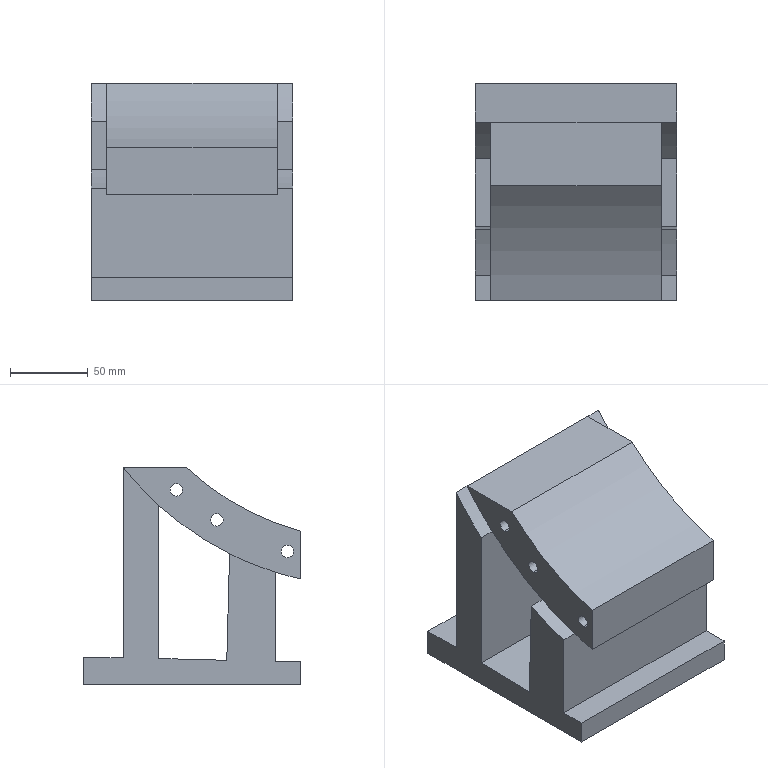Part | SolidWorks | features Cut 4, Extrusion 1, ICE 1 | 1 solid | 29 faces | box 130 x 140 x 140 mm | volume 1223723 mm3 | plane 16 | cylinder 13 | commonest cylinder face diameters 8 x6 406.59 x6 346.59 x1
STEP:
#1=CARTESIAN_POINT('',(120.,98.538,81.808));
#2=VERTEX_POINT('',#1);
#3=CARTESIAN_POINT('',(120.,98.538,89.808));
#4=VERTEX_POINT('',#3);
#5=CARTESIAN_POINT('',(120.,98.538,85.808));
#6=DIRECTION('',(-1.,0.,0.));
#7=DIRECTION('',(0.,0.,1.));
#8=AXIS2_PLACEMENT_3D('',#5,#6,#7);
#9=CIRCLE('',#8,4.);
#10=EDGE_CURVE('',#2,#4,#9,.T.);
#11=ORIENTED_EDGE('',*,*,#10,.F.);
#12=CARTESIAN_POINT('',(10.,98.538,81.808));
#13=VERTEX_POINT('',#12);
#14=CARTESIAN_POINT('',(130.,98.538,81.808));
#15=DIRECTION('',(-1.,0.,0.));
#16=VECTOR('',#15,1000.);
#17=LINE('',#14,#16);
#18=EDGE_CURVE('',#2,#13,#17,.T.);
#19=ORIENTED_EDGE('',*,*,#18,.T.);
#20=CARTESIAN_POINT('',(10.,98.538,89.808));
#21=VERTEX_POINT('',#20);
#22=CARTESIAN_POINT('',(10.,98.538,85.808));
#23=DIRECTION('',(-1.,0.,0.));
#24=DIRECTION('',(0.,0.,1.));
#25=AXIS2_PLACEMENT_3D('',#22,#23,#24);
#26=CIRCLE('',#25,4.);
#27=EDGE_CURVE('',#13,#21,#26,.T.);
#28=ORIENTED_EDGE('',*,*,#27,.T.);
#29=CARTESIAN_POINT('',(130.,98.538,89.808));
#30=DIRECTION('',(-1.,0.,0.));
#31=VECTOR('',#30,1000.);
#32=LINE('',#29,#31);
#33=EDGE_CURVE('',#4,#21,#32,.T.);
#34=ORIENTED_EDGE('',*,*,#33,.F.);
#35=EDGE_LOOP('',(#11,#19,#28,#34));
#36=FACE_OUTER_BOUND('',#35,.T.);
#37=CARTESIAN_POINT('',(130.,98.538,85.808));
#38=DIRECTION('',(-1.,0.,0.));
#39=DIRECTION('',(0.,0.,1.));
#40=AXIS2_PLACEMENT_3D('',#37,#38,#39);
#41=CYLINDRICAL_SURFACE('',#40,4.);
#42=ADVANCED_FACE('',(#36),#41,.F.);
#43=CARTESIAN_POINT('',(120.,143.974,102.133));
#44=VERTEX_POINT('',#43);
#45=CARTESIAN_POINT('',(120.,143.974,110.133));
#46=VERTEX_POINT('',#45);
#47=CARTESIAN_POINT('',(120.,143.974,106.133));
#48=DIRECTION('',(-1.,0.,0.));
#49=DIRECTION('',(0.,0.,1.));
#50=AXIS2_PLACEMENT_3D('',#47,#48,#49);
#51=CIRCLE('',#50,4.);
#52=EDGE_CURVE('',#44,#46,#51,.T.);
#53=ORIENTED_EDGE('',*,*,#52,.F.);
#54=CARTESIAN_POINT('',(10.,143.974,102.133));
#55=VERTEX_POINT('',#54);
#56=CARTESIAN_POINT('',(130.,143.974,102.133));
#57=DIRECTION('',(-1.,0.,0.));
#58=VECTOR('',#57,1000.);
#59=LINE('',#56,#58);
#60=EDGE_CURVE('',#44,#55,#59,.T.);
#61=ORIENTED_EDGE('',*,*,#60,.T.);
#62=CARTESIAN_POINT('',(10.,143.974,110.133));
#63=VERTEX_POINT('',#62);
#64=CARTESIAN_POINT('',(10.,143.974,106.133));
#65=DIRECTION('',(-1.,0.,0.));
#66=DIRECTION('',(0.,0.,1.));
#67=AXIS2_PLACEMENT_3D('',#64,#65,#66);
#68=CIRCLE('',#67,4.);
#69=EDGE_CURVE('',#55,#63,#68,.T.);
#70=ORIENTED_EDGE('',*,*,#69,.T.);
#71=CARTESIAN_POINT('',(130.,143.974,110.133));
#72=DIRECTION('',(-1.,0.,0.));
#73=VECTOR('',#72,1000.);
#74=LINE('',#71,#73);
#75=EDGE_CURVE('',#46,#63,#74,.T.);
#76=ORIENTED_EDGE('',*,*,#75,.F.);
#77=EDGE_LOOP('',(#53,#61,#70,#76));
#78=FACE_OUTER_BOUND('',#77,.T.);
#79=CARTESIAN_POINT('',(130.,143.974,106.133));
#80=DIRECTION('',(-1.,0.,0.));
#81=DIRECTION('',(0.,0.,1.));
#82=AXIS2_PLACEMENT_3D('',#79,#80,#81);
#83=CYLINDRICAL_SURFACE('',#82,4.);
#84=ADVANCED_FACE('',(#78),#83,.F.);
#85=CARTESIAN_POINT('',(120.,170.036,121.519));
#86=VERTEX_POINT('',#85);
#87=CARTESIAN_POINT('',(120.,170.036,129.519));
#88=VERTEX_POINT('',#87);
#89=CARTESIAN_POINT('',(120.,170.036,125.519));
#90=DIRECTION('',(-1.,0.,0.));
#91=DIRECTION('',(0.,0.,1.));
#92=AXIS2_PLACEMENT_3D('',#89,#90,#91);
#93=CIRCLE('',#92,4.);
#94=EDGE_CURVE('',#86,#88,#93,.T.);
#95=ORIENTED_EDGE('',*,*,#94,.F.);
#96=CARTESIAN_POINT('',(10.,170.036,121.519));
#97=VERTEX_POINT('',#96);
#98=CARTESIAN_POINT('',(130.,170.036,121.519));
#99=DIRECTION('',(-1.,0.,0.));
#100=VECTOR('',#99,1000.);
#101=LINE('',#98,#100);
#102=EDGE_CURVE('',#86,#97,#101,.T.);
#103=ORIENTED_EDGE('',*,*,#102,.T.);
#104=CARTESIAN_POINT('',(10.,170.036,129.519));
#105=VERTEX_POINT('',#104);
#106=CARTESIAN_POINT('',(10.,170.036,125.519));
#107=DIRECTION('',(-1.,0.,0.));
#108=DIRECTION('',(0.,0.,1.));
#109=AXIS2_PLACEMENT_3D('',#106,#107,#108);
#110=CIRCLE('',#109,4.);
#111=EDGE_CURVE('',#97,#105,#110,.T.);
#112=ORIENTED_EDGE('',*,*,#111,.T.);
#113=CARTESIAN_POINT('',(130.,170.036,129.519));
#114=DIRECTION('',(-1.,0.,0.));
#115=VECTOR('',#114,1000.);
#116=LINE('',#113,#115);
#117=EDGE_CURVE('',#88,#105,#116,.T.);
#118=ORIENTED_EDGE('',*,*,#117,.F.);
#119=EDGE_LOOP('',(#95,#103,#112,#118));
#120=FACE_OUTER_BOUND('',#119,.T.);
#121=CARTESIAN_POINT('',(130.,170.036,125.519));
#122=DIRECTION('',(-1.,0.,0.));
#123=DIRECTION('',(0.,0.,1.));
#124=AXIS2_PLACEMENT_3D('',#121,#122,#123);
#125=CYLINDRICAL_SURFACE('',#124,4.);
#126=ADVANCED_FACE('',(#120),#125,.F.);
#127=CARTESIAN_POINT('',(10.,90.,68.082));
#128=VERTEX_POINT('',#127);
#129=CARTESIAN_POINT('',(10.,90.,98.982));
#130=VERTEX_POINT('',#129);
#131=CARTESIAN_POINT('',(10.,90.,98.982));
#132=DIRECTION('',(0.,0.,1.));
#133=VECTOR('',#132,1000.);
#134=LINE('',#131,#133);
#135=EDGE_CURVE('',#128,#130,#134,.T.);
#136=ORIENTED_EDGE('',*,*,#135,.F.);
#137=CARTESIAN_POINT('',(120.,90.,68.082));
#138=VERTEX_POINT('',#137);
#139=CARTESIAN_POINT('',(0.,90.,68.082));
#140=DIRECTION('',(1.,0.,0.));
#141=VECTOR('',#140,1000.);
#142=LINE('',#139,#141);
#143=EDGE_CURVE('',#128,#138,#142,.T.);
#144=ORIENTED_EDGE('',*,*,#143,.T.);
#145=CARTESIAN_POINT('',(120.,90.,98.982));
#146=VERTEX_POINT('',#145);
#147=CARTESIAN_POINT('',(120.,90.,98.982));
#148=DIRECTION('',(0.,0.,-1.));
#149=VECTOR('',#148,1000.);
#150=LINE('',#147,#149);
#151=EDGE_CURVE('',#146,#138,#150,.T.);
#152=ORIENTED_EDGE('',*,*,#151,.F.);
#153=CARTESIAN_POINT('',(0.,90.,98.982));
#154=DIRECTION('',(1.,0.,0.));
#155=VECTOR('',#154,1000.);
#156=LINE('',#153,#155);
#157=EDGE_CURVE('',#130,#146,#156,.T.);
#158=ORIENTED_EDGE('',*,*,#157,.F.);
#159=EDGE_LOOP('',(#136,#144,#152,#158));
#160=FACE_OUTER_BOUND('',#159,.T.);
#161=CARTESIAN_POINT('',(0.,90.,10.));
#162=DIRECTION('',(0.,1.,0.));
#163=DIRECTION('',(0.,0.,1.));
#164=AXIS2_PLACEMENT_3D('',#161,#162,#163);
#165=PLANE('',#164);
#166=ADVANCED_FACE('',(#160),#165,.F.);
#167=CARTESIAN_POINT('',(10.,163.653,140.));
#168=VERTEX_POINT('',#167);
#169=CARTESIAN_POINT('',(10.,204.31,140.));
#170=VERTEX_POINT('',#169);
#171=CARTESIAN_POINT('',(10.,163.653,140.));
#172=DIRECTION('',(0.,1.,0.));
#173=VECTOR('',#172,1000.);
#174=LINE('',#171,#173);
#175=EDGE_CURVE('',#168,#170,#174,.T.);
#176=ORIENTED_EDGE('',*,*,#175,.F.);
#177=CARTESIAN_POINT('',(120.,163.653,140.));
#178=VERTEX_POINT('',#177);
#179=CARTESIAN_POINT('',(0.,163.653,140.));
#180=DIRECTION('',(1.,0.,0.));
#181=VECTOR('',#180,1000.);
#182=LINE('',#179,#181);
#183=EDGE_CURVE('',#168,#178,#182,.T.);
#184=ORIENTED_EDGE('',*,*,#183,.T.);
#185=CARTESIAN_POINT('',(120.,204.31,140.));
#186=VERTEX_POINT('',#185);
#187=CARTESIAN_POINT('',(120.,204.31,140.));
#188=DIRECTION('',(0.,-1.,0.));
#189=VECTOR('',#188,1000.);
#190=LINE('',#187,#189);
#191=EDGE_CURVE('',#186,#178,#190,.T.);
#192=ORIENTED_EDGE('',*,*,#191,.F.);
#193=CARTESIAN_POINT('',(0.,204.31,140.));
#194=DIRECTION('',(1.,0.,0.));
#195=VECTOR('',#194,1000.);
#196=LINE('',#193,#195);
#197=EDGE_CURVE('',#170,#186,#196,.T.);
#198=ORIENTED_EDGE('',*,*,#197,.F.);
#199=EDGE_LOOP('',(#176,#184,#192,#198));
#200=FACE_OUTER_BOUND('',#199,.T.);
#201=CARTESIAN_POINT('',(0.,0.,140.));
#202=DIRECTION('',(0.,0.,-1.));
#203=DIRECTION('',(-1.,0.,0.));
#204=AXIS2_PLACEMENT_3D('',#201,#202,#203);
#205=PLANE('',#204);
#206=ADVANCED_FACE('',(#200),#205,.F.);
#207=CARTESIAN_POINT('',(10.,45.043,266.344));
#208=DIRECTION('',(1.,0.,0.));
#209=DIRECTION('',(0.,0.,1.));
#210=AXIS2_PLACEMENT_3D('',#207,#208,#209);
#211=CIRCLE('',#210,173.295);
#212=EDGE_CURVE('',#130,#168,#211,.T.);
#213=ORIENTED_EDGE('',*,*,#212,.F.);
#214=ORIENTED_EDGE('',*,*,#157,.T.);
#215=CARTESIAN_POINT('',(120.,45.043,266.344));
#216=DIRECTION('',(-1.,0.,0.));
#217=DIRECTION('',(0.,0.,-1.));
#218=AXIS2_PLACEMENT_3D('',#215,#216,#217);
#219=CIRCLE('',#218,173.295);
#220=EDGE_CURVE('',#178,#146,#219,.T.);
#221=ORIENTED_EDGE('',*,*,#220,.F.);
#222=ORIENTED_EDGE('',*,*,#183,.F.);
#223=EDGE_LOOP('',(#213,#214,#221,#222));
#224=FACE_OUTER_BOUND('',#223,.T.);
#225=CARTESIAN_POINT('',(0.,45.043,266.344));
#226=DIRECTION('',(1.,0.,0.));
#227=DIRECTION('',(0.,0.,-1.));
#228=AXIS2_PLACEMENT_3D('',#225,#226,#227);
#229=CYLINDRICAL_SURFACE('',#228,173.295);
#230=ADVANCED_FACE('',(#224),#229,.F.);
#231=CARTESIAN_POINT('',(10.,106.264,72.486));
#232=VERTEX_POINT('',#231);
#233=CARTESIAN_POINT('',(10.,45.043,266.344));
#234=DIRECTION('',(-1.,0.,0.));
#235=DIRECTION('',(0.,0.,1.));
#236=AXIS2_PLACEMENT_3D('',#233,#234,#235);
#237=CIRCLE('',#236,203.295);
#238=EDGE_CURVE('',#232,#128,#237,.T.);
#239=ORIENTED_EDGE('',*,*,#238,.F.);
#240=CARTESIAN_POINT('',(120.,106.264,72.486));
#241=VERTEX_POINT('',#240);
#242=CARTESIAN_POINT('',(0.,106.264,72.486));
#243=DIRECTION('',(1.,0.,0.));
#244=VECTOR('',#243,1000.);
#245=LINE('',#242,#244);
#246=EDGE_CURVE('',#232,#241,#245,.T.);
#247=ORIENTED_EDGE('',*,*,#246,.T.);
#248=CARTESIAN_POINT('',(120.,45.043,266.344));
#249=DIRECTION('',(1.,0.,0.));
#250=DIRECTION('',(0.,0.,1.));
#251=AXIS2_PLACEMENT_3D('',#248,#249,#250);
#252=CIRCLE('',#251,203.295);
#253=EDGE_CURVE('',#138,#241,#252,.T.);
#254=ORIENTED_EDGE('',*,*,#253,.F.);
#255=ORIENTED_EDGE('',*,*,#143,.F.);
#256=EDGE_LOOP('',(#239,#247,#254,#255));
#257=FACE_OUTER_BOUND('',#256,.T.);
#258=CARTESIAN_POINT('',(0.,45.043,266.344));
#259=DIRECTION('',(1.,0.,0.));
#260=DIRECTION('',(0.,0.,-1.));
#261=AXIS2_PLACEMENT_3D('',#258,#259,#260);
#262=CYLINDRICAL_SURFACE('',#261,203.295);
#263=ADVANCED_FACE('',(#257),#262,.T.);
#264=CARTESIAN_POINT('',(10.,181.392,115.554));
#265=VERTEX_POINT('',#264);
#266=CARTESIAN_POINT('',(10.,135.773,84.419));
#267=VERTEX_POINT('',#266);
#268=CARTESIAN_POINT('',(10.,45.043,266.344));
#269=DIRECTION('',(-1.,0.,0.));
#270=DIRECTION('',(0.,0.,1.));
#271=AXIS2_PLACEMENT_3D('',#268,#269,#270);
#272=CIRCLE('',#271,203.295);
#273=EDGE_CURVE('',#265,#267,#272,.T.);
#274=ORIENTED_EDGE('',*,*,#273,.F.);
#275=CARTESIAN_POINT('',(120.,181.392,115.554));
#276=VERTEX_POINT('',#275);
#277=CARTESIAN_POINT('',(0.,181.392,115.554));
#278=DIRECTION('',(1.,0.,0.));
#279=VECTOR('',#278,1000.);
#280=LINE('',#277,#279);
#281=EDGE_CURVE('',#265,#276,#280,.T.);
#282=ORIENTED_EDGE('',*,*,#281,.T.);
#283=CARTESIAN_POINT('',(120.,135.773,84.419));
#284=VERTEX_POINT('',#283);
#285=CARTESIAN_POINT('',(120.,45.043,266.344));
#286=DIRECTION('',(-1.,0.,0.));
#287=DIRECTION('',(0.,0.,1.));
#288=AXIS2_PLACEMENT_3D('',#285,#286,#287);
#289=CIRCLE('',#288,203.295);
#290=EDGE_CURVE('',#276,#284,#289,.T.);
#291=ORIENTED_EDGE('',*,*,#290,.T.);
#292=CARTESIAN_POINT('',(0.,135.773,84.419));
#293=DIRECTION('',(1.,0.,0.));
#294=VECTOR('',#293,1000.);
#295=LINE('',#292,#294);
#296=EDGE_CURVE('',#267,#284,#295,.T.);
#297=ORIENTED_EDGE('',*,*,#296,.F.);
#298=EDGE_LOOP('',(#274,#282,#291,#297));
#299=FACE_OUTER_BOUND('',#298,.T.);
#300=CARTESIAN_POINT('',(0.,45.043,266.344));
#301=DIRECTION('',(1.,0.,0.));
#302=DIRECTION('',(0.,0.,-1.));
#303=AXIS2_PLACEMENT_3D('',#300,#301,#302);
#304=CYLINDRICAL_SURFACE('',#303,203.295);
#305=ADVANCED_FACE('',(#299),#304,.T.);
#306=CARTESIAN_POINT('',(0.,230.,17.408));
#307=VERTEX_POINT('',#306);
#308=CARTESIAN_POINT('',(0.,230.,0.));
#309=VERTEX_POINT('',#308);
#310=CARTESIAN_POINT('',(0.,230.,10.));
#311=DIRECTION('',(0.,0.,-1.));
#312=VECTOR('',#311,1000.);
#313=LINE('',#310,#312);
#314=EDGE_CURVE('',#307,#309,#313,.T.);
#315=ORIENTED_EDGE('',*,*,#314,.F.);
#316=CARTESIAN_POINT('',(130.,230.,17.408));
#317=VERTEX_POINT('',#316);
#318=CARTESIAN_POINT('',(0.,230.,17.408));
#319=DIRECTION('',(1.,0.,0.));
#320=VECTOR('',#319,1000.);
#321=LINE('',#318,#320);
#322=EDGE_CURVE('',#307,#317,#321,.T.);
#323=ORIENTED_EDGE('',*,*,#322,.T.);
#324=CARTESIAN_POINT('',(130.,230.,0.));
#325=VERTEX_POINT('',#324);
#326=CARTESIAN_POINT('',(130.,230.,10.));
#327=DIRECTION('',(0.,0.,-1.));
#328=VECTOR('',#327,1000.);
#329=LINE('',#326,#328);
#330=EDGE_CURVE('',#317,#325,#329,.T.);
#331=ORIENTED_EDGE('',*,*,#330,.T.);
#332=CARTESIAN_POINT('',(130.,230.,0.));
#333=DIRECTION('',(-1.,0.,0.));
#334=VECTOR('',#333,1000.);
#335=LINE('',#332,#334);
#336=EDGE_CURVE('',#325,#309,#335,.T.);
#337=ORIENTED_EDGE('',*,*,#336,.T.);
#338=EDGE_LOOP('',(#315,#323,#331,#337));
#339=FACE_OUTER_BOUND('',#338,.T.);
#340=CARTESIAN_POINT('',(130.,230.,10.));
#341=DIRECTION('',(0.,-1.,0.));
#342=DIRECTION('',(0.,0.,-1.));
#343=AXIS2_PLACEMENT_3D('',#340,#341,#342);
#344=PLANE('',#343);
#345=ADVANCED_FACE('',(#339),#344,.F.);
#346=CARTESIAN_POINT('',(0.,106.264,14.84));
#347=VERTEX_POINT('',#346);
#348=CARTESIAN_POINT('',(0.,106.264,72.486));
#349=VERTEX_POINT('',#348);
#350=CARTESIAN_POINT('',(0.,106.264,14.84));
#351=DIRECTION('',(0.,0.,1.));
#352=VECTOR('',#351,1000.);
#353=LINE('',#350,#352);
#354=EDGE_CURVE('',#347,#349,#353,.T.);
#355=ORIENTED_EDGE('',*,*,#354,.T.);
#356=CARTESIAN_POINT('',(0.,135.773,84.419));
#357=VERTEX_POINT('',#356);
#358=CARTESIAN_POINT('',(0.,45.043,266.344));
#359=DIRECTION('',(-1.,0.,0.));
#360=DIRECTION('',(0.,0.,1.));
#361=AXIS2_PLACEMENT_3D('',#358,#359,#360);
#362=CIRCLE('',#361,203.295);
#363=EDGE_CURVE('',#357,#349,#362,.T.);
#364=ORIENTED_EDGE('',*,*,#363,.F.);
#365=CARTESIAN_POINT('',(0.,137.574,15.66));
#366=VERTEX_POINT('',#365);
#367=CARTESIAN_POINT('',(0.,137.574,15.66));
#368=DIRECTION('',(0.,0.02618,-0.9997));
#369=VECTOR('',#368,1000.);
#370=LINE('',#367,#369);
#371=EDGE_CURVE('',#357,#366,#370,.T.);
#372=ORIENTED_EDGE('',*,*,#371,.T.);
#373=CARTESIAN_POINT('',(0.,181.392,16.808));
#374=VERTEX_POINT('',#373);
#375=CARTESIAN_POINT('',(0.,181.392,16.808));
#376=DIRECTION('',(0.,0.9997,0.02618));
#377=VECTOR('',#376,1000.);
#378=LINE('',#375,#377);
#379=EDGE_CURVE('',#366,#374,#378,.T.);
#380=ORIENTED_EDGE('',*,*,#379,.T.);
#381=CARTESIAN_POINT('',(0.,181.392,115.554));
#382=VERTEX_POINT('',#381);
#383=CARTESIAN_POINT('',(0.,181.392,16.808));
#384=DIRECTION('',(0.,0.,1.));
#385=VECTOR('',#384,1000.);
#386=LINE('',#383,#385);
#387=EDGE_CURVE('',#374,#382,#386,.T.);
#388=ORIENTED_EDGE('',*,*,#387,.T.);
#389=CARTESIAN_POINT('',(0.,204.31,140.));
#390=VERTEX_POINT('',#389);
#391=CARTESIAN_POINT('',(0.,45.043,266.344));
#392=DIRECTION('',(-1.,0.,0.));
#393=DIRECTION('',(0.,0.,1.));
#394=AXIS2_PLACEMENT_3D('',#391,#392,#393);
#395=CIRCLE('',#394,203.295);
#396=EDGE_CURVE('',#390,#382,#395,.T.);
#397=ORIENTED_EDGE('',*,*,#396,.F.);
#398=CARTESIAN_POINT('',(0.,204.31,17.408));
#399=VERTEX_POINT('',#398);
#400=CARTESIAN_POINT('',(0.,204.31,140.));
#401=DIRECTION('',(0.,0.,-1.));
#402=VECTOR('',#401,1000.);
#403=LINE('',#400,#402);
#404=EDGE_CURVE('',#390,#399,#403,.T.);
#405=ORIENTED_EDGE('',*,*,#404,.T.);
#406=CARTESIAN_POINT('',(0.,204.31,17.408));
#407=DIRECTION('',(0.,1.,0.));
#408=VECTOR('',#407,1000.);
#409=LINE('',#406,#408);
#410=EDGE_CURVE('',#399,#307,#409,.T.);
#411=ORIENTED_EDGE('',*,*,#410,.T.);
#412=ORIENTED_EDGE('',*,*,#314,.T.);
#413=CARTESIAN_POINT('',(0.,90.,0.));
#414=VERTEX_POINT('',#413);
#415=CARTESIAN_POINT('',(0.,230.,0.));
#416=DIRECTION('',(0.,-1.,0.));
#417=VECTOR('',#416,1000.);
#418=LINE('',#415,#417);
#419=EDGE_CURVE('',#309,#414,#418,.T.);
#420=ORIENTED_EDGE('',*,*,#419,.T.);
#421=CARTESIAN_POINT('',(0.,90.,14.84));
#422=VERTEX_POINT('',#421);
#423=CARTESIAN_POINT('',(0.,90.,10.));
#424=DIRECTION('',(0.,0.,-1.));
#425=VECTOR('',#424,1000.);
#426=LINE('',#423,#425);
#427=EDGE_CURVE('',#422,#414,#426,.T.);
#428=ORIENTED_EDGE('',*,*,#427,.F.);
#429=CARTESIAN_POINT('',(0.,90.,14.84));
#430=DIRECTION('',(0.,1.,0.));
#431=VECTOR('',#430,1000.);
#432=LINE('',#429,#431);
#433=EDGE_CURVE('',#422,#347,#432,.T.);
#434=ORIENTED_EDGE('',*,*,#433,.T.);
#435=EDGE_LOOP('',(#355,#364,#372,#380,#388,#397,#405,#411,#412,#420,#428,#434));
#436=FACE_OUTER_BOUND('',#435,.T.);
#437=CARTESIAN_POINT('',(0.,230.,10.));
#438=DIRECTION('',(1.,0.,0.));
#439=DIRECTION('',(0.,0.,-1.));
#440=AXIS2_PLACEMENT_3D('',#437,#438,#439);
#441=PLANE('',#440);
#442=ADVANCED_FACE('',(#436),#441,.F.);
#443=CARTESIAN_POINT('',(130.,90.,14.84));
#444=VERTEX_POINT('',#443);
#445=CARTESIAN_POINT('',(130.,90.,0.));
#446=VERTEX_POINT('',#445);
#447=CARTESIAN_POINT('',(130.,90.,10.));
#448=DIRECTION('',(0.,0.,-1.));
#449=VECTOR('',#448,1000.);
#450=LINE('',#447,#449);
#451=EDGE_CURVE('',#444,#446,#450,.T.);
#452=ORIENTED_EDGE('',*,*,#451,.F.);
#453=CARTESIAN_POINT('',(0.,90.,14.84));
#454=DIRECTION('',(1.,0.,0.));
#455=VECTOR('',#454,1000.);
#456=LINE('',#453,#455);
#457=EDGE_CURVE('',#422,#444,#456,.T.);
#458=ORIENTED_EDGE('',*,*,#457,.F.);
#459=ORIENTED_EDGE('',*,*,#427,.T.);
#460=CARTESIAN_POINT('',(0.,90.,0.));
#461=DIRECTION('',(1.,0.,0.));
#462=VECTOR('',#461,1000.);
#463=LINE('',#460,#462);
#464=EDGE_CURVE('',#414,#446,#463,.T.);
#465=ORIENTED_EDGE('',*,*,#464,.T.);
#466=EDGE_LOOP('',(#452,#458,#459,#465));
#467=FACE_OUTER_BOUND('',#466,.T.);
#468=CARTESIAN_POINT('',(0.,90.,10.));
#469=DIRECTION('',(0.,1.,0.));
#470=DIRECTION('',(0.,0.,1.));
#471=AXIS2_PLACEMENT_3D('',#468,#469,#470);
#472=PLANE('',#471);
#473=ADVANCED_FACE('',(#467),#472,.F.);
#474=CARTESIAN_POINT('',(130.,204.31,17.408));
#475=VERTEX_POINT('',#474);
#476=CARTESIAN_POINT('',(130.,204.31,140.));
#477=VERTEX_POINT('',#476);
#478=CARTESIAN_POINT('',(130.,204.31,10.));
#479=DIRECTION('',(0.,0.,1.));
#480=VECTOR('',#479,1000.);
#481=LINE('',#478,#480);
#482=EDGE_CURVE('',#475,#477,#481,.T.);
#483=ORIENTED_EDGE('',*,*,#482,.T.);
#484=CARTESIAN_POINT('',(130.,181.392,115.554));
#485=VERTEX_POINT('',#484);
#486=CARTESIAN_POINT('',(130.,45.043,266.344));
#487=DIRECTION('',(-1.,0.,0.));
#488=DIRECTION('',(0.,0.,1.));
#489=AXIS2_PLACEMENT_3D('',#486,#487,#488);
#490=CIRCLE('',#489,203.295);
#491=EDGE_CURVE('',#477,#485,#490,.T.);
#492=ORIENTED_EDGE('',*,*,#491,.T.);
#493=CARTESIAN_POINT('',(130.,181.392,16.808));
#494=VERTEX_POINT('',#493);
#495=CARTESIAN_POINT('',(130.,181.392,10.));
#496=DIRECTION('',(0.,0.,-1.));
#497=VECTOR('',#496,1000.);
#498=LINE('',#495,#497);
#499=EDGE_CURVE('',#485,#494,#498,.T.);
#500=ORIENTED_EDGE('',*,*,#499,.T.);
#501=CARTESIAN_POINT('',(130.,137.574,15.66));
#502=VERTEX_POINT('',#501);
#503=CARTESIAN_POINT('',(130.,89.884,14.411));
#504=DIRECTION('',(0.,-0.9997,-0.02618));
#505=VECTOR('',#504,1000.);
#506=LINE('',#503,#505);
#507=EDGE_CURVE('',#494,#502,#506,.T.);
#508=ORIENTED_EDGE('',*,*,#507,.T.);
#509=CARTESIAN_POINT('',(130.,135.773,84.419));
#510=VERTEX_POINT('',#509);
#511=CARTESIAN_POINT('',(130.,137.69,11.249));
#512=DIRECTION('',(0.,-0.02618,0.9997));
#513=VECTOR('',#512,1000.);
#514=LINE('',#511,#513);
#515=EDGE_CURVE('',#502,#510,#514,.T.);
#516=ORIENTED_EDGE('',*,*,#515,.T.);
#517=CARTESIAN_POINT('',(130.,106.264,72.486));
#518=VERTEX_POINT('',#517);
#519=CARTESIAN_POINT('',(130.,45.043,266.344));
#520=DIRECTION('',(-1.,0.,0.));
#521=DIRECTION('',(0.,0.,1.));
#522=AXIS2_PLACEMENT_3D('',#519,#520,#521);
#523=CIRCLE('',#522,203.295);
#524=EDGE_CURVE('',#510,#518,#523,.T.);
#525=ORIENTED_EDGE('',*,*,#524,.T.);
#526=CARTESIAN_POINT('',(130.,106.264,14.84));
#527=VERTEX_POINT('',#526);
#528=CARTESIAN_POINT('',(130.,106.264,10.));
#529=DIRECTION('',(0.,0.,-1.));
#530=VECTOR('',#529,1000.);
#531=LINE('',#528,#530);
#532=EDGE_CURVE('',#518,#527,#531,.T.);
#533=ORIENTED_EDGE('',*,*,#532,.T.);
#534=CARTESIAN_POINT('',(130.,90.,14.84));
#535=DIRECTION('',(0.,-1.,0.));
#536=VECTOR('',#535,1000.);
#537=LINE('',#534,#536);
#538=EDGE_CURVE('',#527,#444,#537,.T.);
#539=ORIENTED_EDGE('',*,*,#538,.T.);
#540=ORIENTED_EDGE('',*,*,#451,.T.);
#541=CARTESIAN_POINT('',(130.,90.,0.));
#542=DIRECTION('',(0.,1.,0.));
#543=VECTOR('',#542,1000.);
#544=LINE('',#541,#543);
#545=EDGE_CURVE('',#446,#325,#544,.T.);
#546=ORIENTED_EDGE('',*,*,#545,.T.);
#547=ORIENTED_EDGE('',*,*,#330,.F.);
#548=CARTESIAN_POINT('',(130.,90.,17.408));
#549=DIRECTION('',(0.,-1.,0.));
#550=VECTOR('',#549,1000.);
#551=LINE('',#548,#550);
#552=EDGE_CURVE('',#317,#475,#551,.T.);
#553=ORIENTED_EDGE('',*,*,#552,.T.);
#554=EDGE_LOOP('',(#483,#492,#500,#508,#516,#525,#533,#539,#540,#546,#547,#553));
#555=FACE_OUTER_BOUND('',#554,.T.);
#556=CARTESIAN_POINT('',(130.,90.,10.));
#557=DIRECTION('',(-1.,0.,0.));
#558=DIRECTION('',(0.,0.,1.));
#559=AXIS2_PLACEMENT_3D('',#556,#557,#558);
#560=PLANE('',#559);
#561=ADVANCED_FACE('',(#555),#560,.F.);
#562=ORIENTED_EDGE('',*,*,#336,.F.);
#563=ORIENTED_EDGE('',*,*,#545,.F.);
#564=ORIENTED_EDGE('',*,*,#464,.F.);
#565=ORIENTED_EDGE('',*,*,#419,.F.);
#566=EDGE_LOOP('',(#562,#563,#564,#565));
#567=FACE_OUTER_BOUND('',#566,.T.);
#568=CARTESIAN_POINT('',(0.,0.,0.));
#569=DIRECTION('',(0.,0.,1.));
#570=DIRECTION('',(1.,0.,0.));
#571=AXIS2_PLACEMENT_3D('',#568,#569,#570);
#572=PLANE('',#571);
#573=ADVANCED_FACE('',(#567),#572,.F.);
#574=ORIENTED_EDGE('',*,*,#322,.F.);
#575=ORIENTED_EDGE('',*,*,#410,.F.);
#576=CARTESIAN_POINT('',(0.,204.31,17.408));
#577=DIRECTION('',(1.,0.,0.));
#578=VECTOR('',#577,1000.);
#579=LINE('',#576,#578);
#580=EDGE_CURVE('',#399,#475,#579,.T.);
#581=ORIENTED_EDGE('',*,*,#580,.T.);
#582=ORIENTED_EDGE('',*,*,#552,.F.);
#583=EDGE_LOOP('',(#574,#575,#581,#582));
#584=FACE_OUTER_BOUND('',#583,.T.);
#585=CARTESIAN_POINT('',(0.,204.31,17.408));
#586=DIRECTION('',(0.,0.,-1.));
#587=DIRECTION('',(-1.,0.,0.));
#588=AXIS2_PLACEMENT_3D('',#585,#586,#587);
#589=PLANE('',#588);
#590=ADVANCED_FACE('',(#584),#589,.F.);
#591=ORIENTED_EDGE('',*,*,#580,.F.);
#592=ORIENTED_EDGE('',*,*,#404,.F.);
#593=CARTESIAN_POINT('',(0.,204.31,140.));
#594=DIRECTION('',(1.,0.,0.));
#595=VECTOR('',#594,1000.);
#596=LINE('',#593,#595);
#597=EDGE_CURVE('',#390,#170,#596,.T.);
#598=ORIENTED_EDGE('',*,*,#597,.T.);
#599=ORIENTED_EDGE('',*,*,#197,.T.);
#600=CARTESIAN_POINT('',(120.,204.31,140.));
#601=DIRECTION('',(1.,0.,0.));
#602=VECTOR('',#601,1000.);
#603=LINE('',#600,#602);
#604=EDGE_CURVE('',#186,#477,#603,.T.);
#605=ORIENTED_EDGE('',*,*,#604,.T.);
#606=ORIENTED_EDGE('',*,*,#482,.F.);
#607=EDGE_LOOP('',(#591,#592,#598,#599,#605,#606));
#608=FACE_OUTER_BOUND('',#607,.T.);
#609=CARTESIAN_POINT('',(0.,204.31,140.));
#610=DIRECTION('',(0.,-1.,0.));
#611=DIRECTION('',(0.,0.,-1.));
#612=AXIS2_PLACEMENT_3D('',#609,#610,#611);
#613=PLANE('',#612);
#614=ADVANCED_FACE('',(#608),#613,.F.);
#615=CARTESIAN_POINT('',(0.,106.264,72.486));
#616=DIRECTION('',(1.,0.,0.));
#617=VECTOR('',#616,1000.);
#618=LINE('',#615,#617);
#619=EDGE_CURVE('',#349,#232,#618,.T.);
#620=ORIENTED_EDGE('',*,*,#619,.F.);
#621=ORIENTED_EDGE('',*,*,#354,.F.);
#622=CARTESIAN_POINT('',(0.,106.264,14.84));
#623=DIRECTION('',(1.,0.,0.));
#624=VECTOR('',#623,1000.);
#625=LINE('',#622,#624);
#626=EDGE_CURVE('',#347,#527,#625,.T.);
#627=ORIENTED_EDGE('',*,*,#626,.T.);
#628=ORIENTED_EDGE('',*,*,#532,.F.);
#629=CARTESIAN_POINT('',(120.,106.264,72.486));
#630=DIRECTION('',(-1.,0.,0.));
#631=VECTOR('',#630,1000.);
#632=LINE('',#629,#631);
#633=EDGE_CURVE('',#518,#241,#632,.T.);
#634=ORIENTED_EDGE('',*,*,#633,.T.);
#635=ORIENTED_EDGE('',*,*,#246,.F.);
#636=EDGE_LOOP('',(#620,#621,#627,#628,#634,#635));
#637=FACE_OUTER_BOUND('',#636,.T.);
#638=CARTESIAN_POINT('',(0.,106.264,14.84));
#639=DIRECTION('',(0.,1.,0.));
#640=DIRECTION('',(0.,0.,1.));
#641=AXIS2_PLACEMENT_3D('',#638,#639,#640);
#642=PLANE('',#641);
#643=ADVANCED_FACE('',(#637),#642,.F.);
#644=ORIENTED_EDGE('',*,*,#626,.F.);
#645=ORIENTED_EDGE('',*,*,#433,.F.);
#646=ORIENTED_EDGE('',*,*,#457,.T.);
#647=ORIENTED_EDGE('',*,*,#538,.F.);
#648=EDGE_LOOP('',(#644,#645,#646,#647));
#649=FACE_OUTER_BOUND('',#648,.T.);
#650=CARTESIAN_POINT('',(0.,90.,14.84));
#651=DIRECTION('',(0.,0.,-1.));
#652=DIRECTION('',(-1.,0.,0.));
#653=AXIS2_PLACEMENT_3D('',#650,#651,#652);
#654=PLANE('',#653);
#655=ADVANCED_FACE('',(#649),#654,.F.);
#656=CARTESIAN_POINT('',(0.,181.392,115.554));
#657=DIRECTION('',(1.,0.,0.));
#658=VECTOR('',#657,1000.);
#659=LINE('',#656,#658);
#660=EDGE_CURVE('',#382,#265,#659,.T.);
#661=ORIENTED_EDGE('',*,*,#660,.F.);
#662=ORIENTED_EDGE('',*,*,#387,.F.);
#663=CARTESIAN_POINT('',(0.,181.392,16.808));
#664=DIRECTION('',(1.,0.,0.));
#665=VECTOR('',#664,1000.);
#666=LINE('',#663,#665);
#667=EDGE_CURVE('',#374,#494,#666,.T.);
#668=ORIENTED_EDGE('',*,*,#667,.T.);
#669=ORIENTED_EDGE('',*,*,#499,.F.);
#670=CARTESIAN_POINT('',(0.,181.392,115.554));
#671=DIRECTION('',(1.,0.,0.));
#672=VECTOR('',#671,1000.);
#673=LINE('',#670,#672);
#674=EDGE_CURVE('',#276,#485,#673,.T.);
#675=ORIENTED_EDGE('',*,*,#674,.F.);
#676=ORIENTED_EDGE('',*,*,#281,.F.);
#677=EDGE_LOOP('',(#661,#662,#668,#669,#675,#676));
#678=FACE_OUTER_BOUND('',#677,.T.);
#679=CARTESIAN_POINT('',(0.,181.392,16.808));
#680=DIRECTION('',(0.,1.,0.));
#681=DIRECTION('',(0.,0.,1.));
#682=AXIS2_PLACEMENT_3D('',#679,#680,#681);
#683=PLANE('',#682);
#684=ADVANCED_FACE('',(#678),#683,.F.);
#685=ORIENTED_EDGE('',*,*,#667,.F.);
#686=ORIENTED_EDGE('',*,*,#379,.F.);
#687=CARTESIAN_POINT('',(0.,137.574,15.66));
#688=DIRECTION('',(1.,0.,0.));
#689=VECTOR('',#688,1000.);
#690=LINE('',#687,#689);
#691=EDGE_CURVE('',#366,#502,#690,.T.);
#692=ORIENTED_EDGE('',*,*,#691,.T.);
#693=ORIENTED_EDGE('',*,*,#507,.F.);
#694=EDGE_LOOP('',(#685,#686,#692,#693));
#695=FACE_OUTER_BOUND('',#694,.T.);
#696=CARTESIAN_POINT('',(0.,181.392,16.808));
#697=DIRECTION('',(0.,0.02618,-0.9997));
#698=DIRECTION('',(0.,0.9997,0.02618));
#699=AXIS2_PLACEMENT_3D('',#696,#697,#698);
#700=PLANE('',#699);
#701=ADVANCED_FACE('',(#695),#700,.F.);
#702=ORIENTED_EDGE('',*,*,#691,.F.);
#703=ORIENTED_EDGE('',*,*,#371,.F.);
#704=CARTESIAN_POINT('',(0.,135.773,84.419));
#705=DIRECTION('',(1.,0.,0.));
#706=VECTOR('',#705,1000.);
#707=LINE('',#704,#706);
#708=EDGE_CURVE('',#357,#267,#707,.T.);
#709=ORIENTED_EDGE('',*,*,#708,.T.);
#710=ORIENTED_EDGE('',*,*,#296,.T.);
#711=CARTESIAN_POINT('',(0.,135.773,84.419));
#712=DIRECTION('',(1.,0.,0.));
#713=VECTOR('',#712,1000.);
#714=LINE('',#711,#713);
#715=EDGE_CURVE('',#284,#510,#714,.T.);
#716=ORIENTED_EDGE('',*,*,#715,.T.);
#717=ORIENTED_EDGE('',*,*,#515,.F.);
#718=EDGE_LOOP('',(#702,#703,#709,#710,#716,#717));
#719=FACE_OUTER_BOUND('',#718,.T.);
#720=CARTESIAN_POINT('',(0.,137.574,15.66));
#721=DIRECTION('',(0.,-0.9997,-0.02618));
#722=DIRECTION('',(0.,0.02618,-0.9997));
#723=AXIS2_PLACEMENT_3D('',#720,#721,#722);
#724=PLANE('',#723);
#725=ADVANCED_FACE('',(#719),#724,.F.);
#726=ORIENTED_EDGE('',*,*,#604,.F.);
#727=CARTESIAN_POINT('',(120.,45.043,266.344));
#728=DIRECTION('',(1.,0.,0.));
#729=DIRECTION('',(0.,0.,1.));
#730=AXIS2_PLACEMENT_3D('',#727,#728,#729);
#731=CIRCLE('',#730,203.295);
#732=EDGE_CURVE('',#276,#186,#731,.T.);
#733=ORIENTED_EDGE('',*,*,#732,.F.);
#734=ORIENTED_EDGE('',*,*,#674,.T.);
#735=ORIENTED_EDGE('',*,*,#491,.F.);
#736=EDGE_LOOP('',(#726,#733,#734,#735));
#737=FACE_OUTER_BOUND('',#736,.T.);
#738=CARTESIAN_POINT('',(120.,45.043,266.344));
#739=DIRECTION('',(1.,0.,0.));
#740=DIRECTION('',(0.,0.,-1.));
#741=AXIS2_PLACEMENT_3D('',#738,#739,#740);
#742=CYLINDRICAL_SURFACE('',#741,203.295);
#743=ADVANCED_FACE('',(#737),#742,.F.);
#744=ORIENTED_EDGE('',*,*,#524,.F.);
#745=ORIENTED_EDGE('',*,*,#715,.F.);
#746=CARTESIAN_POINT('',(120.,45.043,266.344));
#747=DIRECTION('',(1.,0.,0.));
#748=DIRECTION('',(0.,0.,1.));
#749=AXIS2_PLACEMENT_3D('',#746,#747,#748);
#750=CIRCLE('',#749,203.295);
#751=EDGE_CURVE('',#241,#284,#750,.T.);
#752=ORIENTED_EDGE('',*,*,#751,.F.);
#753=ORIENTED_EDGE('',*,*,#633,.F.);
#754=EDGE_LOOP('',(#744,#745,#752,#753));
#755=FACE_OUTER_BOUND('',#754,.T.);
#756=CARTESIAN_POINT('',(120.,45.043,266.344));
#757=DIRECTION('',(1.,0.,0.));
#758=DIRECTION('',(0.,0.,-1.));
#759=AXIS2_PLACEMENT_3D('',#756,#757,#758);
#760=CYLINDRICAL_SURFACE('',#759,203.295);
#761=ADVANCED_FACE('',(#755),#760,.F.);
#762=CARTESIAN_POINT('',(120.,98.538,85.808));
#763=DIRECTION('',(-1.,0.,0.));
#764=DIRECTION('',(0.,0.,1.));
#765=AXIS2_PLACEMENT_3D('',#762,#763,#764);
#766=CIRCLE('',#765,4.);
#767=EDGE_CURVE('',#4,#2,#766,.T.);
#768=ORIENTED_EDGE('',*,*,#767,.T.);
#769=ORIENTED_EDGE('',*,*,#10,.T.);
#770=EDGE_LOOP('',(#768,#769));
#771=FACE_BOUND('',#770,.T.);
#772=CARTESIAN_POINT('',(120.,143.974,106.133));
#773=DIRECTION('',(-1.,0.,0.));
#774=DIRECTION('',(0.,0.,1.));
#775=AXIS2_PLACEMENT_3D('',#772,#773,#774);
#776=CIRCLE('',#775,4.);
#777=EDGE_CURVE('',#46,#44,#776,.T.);
#778=ORIENTED_EDGE('',*,*,#777,.T.);
#779=ORIENTED_EDGE('',*,*,#52,.T.);
#780=EDGE_LOOP('',(#778,#779));
#781=FACE_BOUND('',#780,.T.);
#782=CARTESIAN_POINT('',(120.,170.036,125.519));
#783=DIRECTION('',(-1.,0.,0.));
#784=DIRECTION('',(0.,0.,1.));
#785=AXIS2_PLACEMENT_3D('',#782,#783,#784);
#786=CIRCLE('',#785,4.);
#787=EDGE_CURVE('',#88,#86,#786,.T.);
#788=ORIENTED_EDGE('',*,*,#787,.T.);
#789=ORIENTED_EDGE('',*,*,#94,.T.);
#790=EDGE_LOOP('',(#788,#789));
#791=FACE_BOUND('',#790,.T.);
#792=ORIENTED_EDGE('',*,*,#253,.T.);
#793=ORIENTED_EDGE('',*,*,#751,.T.);
#794=ORIENTED_EDGE('',*,*,#290,.F.);
#795=ORIENTED_EDGE('',*,*,#732,.T.);
#796=ORIENTED_EDGE('',*,*,#191,.T.);
#797=ORIENTED_EDGE('',*,*,#220,.T.);
#798=ORIENTED_EDGE('',*,*,#151,.T.);
#799=EDGE_LOOP('',(#792,#793,#794,#795,#796,#797,#798));
#800=FACE_OUTER_BOUND('',#799,.T.);
#801=CARTESIAN_POINT('',(120.,45.043,266.344));
#802=DIRECTION('',(-1.,0.,0.));
#803=DIRECTION('',(0.,0.,1.));
#804=AXIS2_PLACEMENT_3D('',#801,#802,#803);
#805=PLANE('',#804);
#806=ADVANCED_FACE('',(#771,#781,#791,#800),#805,.F.);
#807=CARTESIAN_POINT('',(10.,45.043,266.344));
#808=DIRECTION('',(-1.,0.,0.));
#809=DIRECTION('',(0.,0.,1.));
#810=AXIS2_PLACEMENT_3D('',#807,#808,#809);
#811=CIRCLE('',#810,203.295);
#812=EDGE_CURVE('',#267,#232,#811,.T.);
#813=ORIENTED_EDGE('',*,*,#812,.F.);
#814=ORIENTED_EDGE('',*,*,#708,.F.);
#815=ORIENTED_EDGE('',*,*,#363,.T.);
#816=ORIENTED_EDGE('',*,*,#619,.T.);
#817=EDGE_LOOP('',(#813,#814,#815,#816));
#818=FACE_OUTER_BOUND('',#817,.T.);
#819=CARTESIAN_POINT('',(10.,45.043,266.344));
#820=DIRECTION('',(-1.,0.,0.));
#821=DIRECTION('',(0.,0.,1.));
#822=AXIS2_PLACEMENT_3D('',#819,#820,#821);
#823=CYLINDRICAL_SURFACE('',#822,203.295);
#824=ADVANCED_FACE('',(#818),#823,.F.);
#825=CARTESIAN_POINT('',(10.,45.043,266.344));
#826=DIRECTION('',(-1.,0.,0.));
#827=DIRECTION('',(0.,0.,1.));
#828=AXIS2_PLACEMENT_3D('',#825,#826,#827);
#829=CIRCLE('',#828,203.295);
#830=EDGE_CURVE('',#170,#265,#829,.T.);
#831=ORIENTED_EDGE('',*,*,#830,.F.);
#832=ORIENTED_EDGE('',*,*,#597,.F.);
#833=ORIENTED_EDGE('',*,*,#396,.T.);
#834=ORIENTED_EDGE('',*,*,#660,.T.);
#835=EDGE_LOOP('',(#831,#832,#833,#834));
#836=FACE_OUTER_BOUND('',#835,.T.);
#837=CARTESIAN_POINT('',(10.,45.043,266.344));
#838=DIRECTION('',(-1.,0.,0.));
#839=DIRECTION('',(0.,0.,1.));
#840=AXIS2_PLACEMENT_3D('',#837,#838,#839);
#841=CYLINDRICAL_SURFACE('',#840,203.295);
#842=ADVANCED_FACE('',(#836),#841,.F.);
#843=CARTESIAN_POINT('',(10.,98.538,85.808));
#844=DIRECTION('',(-1.,0.,0.));
#845=DIRECTION('',(0.,0.,1.));
#846=AXIS2_PLACEMENT_3D('',#843,#844,#845);
#847=CIRCLE('',#846,4.);
#848=EDGE_CURVE('',#21,#13,#847,.T.);
#849=ORIENTED_EDGE('',*,*,#848,.F.);
#850=ORIENTED_EDGE('',*,*,#27,.F.);
#851=EDGE_LOOP('',(#849,#850));
#852=FACE_BOUND('',#851,.T.);
#853=CARTESIAN_POINT('',(10.,143.974,106.133));
#854=DIRECTION('',(-1.,0.,0.));
#855=DIRECTION('',(0.,0.,1.));
#856=AXIS2_PLACEMENT_3D('',#853,#854,#855);
#857=CIRCLE('',#856,4.);
#858=EDGE_CURVE('',#63,#55,#857,.T.);
#859=ORIENTED_EDGE('',*,*,#858,.F.);
#860=ORIENTED_EDGE('',*,*,#69,.F.);
#861=EDGE_LOOP('',(#859,#860));
#862=FACE_BOUND('',#861,.T.);
#863=CARTESIAN_POINT('',(10.,170.036,125.519));
#864=DIRECTION('',(-1.,0.,0.));
#865=DIRECTION('',(0.,0.,1.));
#866=AXIS2_PLACEMENT_3D('',#863,#864,#865);
#867=CIRCLE('',#866,4.);
#868=EDGE_CURVE('',#105,#97,#867,.T.);
#869=ORIENTED_EDGE('',*,*,#868,.F.);
#870=ORIENTED_EDGE('',*,*,#111,.F.);
#871=EDGE_LOOP('',(#869,#870));
#872=FACE_BOUND('',#871,.T.);
#873=ORIENTED_EDGE('',*,*,#212,.T.);
#874=ORIENTED_EDGE('',*,*,#175,.T.);
#875=ORIENTED_EDGE('',*,*,#830,.T.);
#876=ORIENTED_EDGE('',*,*,#273,.T.);
#877=ORIENTED_EDGE('',*,*,#812,.T.);
#878=ORIENTED_EDGE('',*,*,#238,.T.);
#879=ORIENTED_EDGE('',*,*,#135,.T.);
#880=EDGE_LOOP('',(#873,#874,#875,#876,#877,#878,#879));
#881=FACE_OUTER_BOUND('',#880,.T.);
#882=CARTESIAN_POINT('',(10.,45.043,266.344));
#883=DIRECTION('',(-1.,0.,0.));
#884=DIRECTION('',(0.,0.,1.));
#885=AXIS2_PLACEMENT_3D('',#882,#883,#884);
#886=PLANE('',#885);
#887=ADVANCED_FACE('',(#852,#862,#872,#881),#886,.T.);
#888=ORIENTED_EDGE('',*,*,#102,.F.);
#889=ORIENTED_EDGE('',*,*,#787,.F.);
#890=ORIENTED_EDGE('',*,*,#117,.T.);
#891=ORIENTED_EDGE('',*,*,#868,.T.);
#892=EDGE_LOOP('',(#888,#889,#890,#891));
#893=FACE_OUTER_BOUND('',#892,.T.);
#894=CARTESIAN_POINT('',(130.,170.036,125.519));
#895=DIRECTION('',(-1.,0.,0.));
#896=DIRECTION('',(0.,0.,1.));
#897=AXIS2_PLACEMENT_3D('',#894,#895,#896);
#898=CYLINDRICAL_SURFACE('',#897,4.);
#899=ADVANCED_FACE('',(#893),#898,.F.);
#900=ORIENTED_EDGE('',*,*,#60,.F.);
#901=ORIENTED_EDGE('',*,*,#777,.F.);
#902=ORIENTED_EDGE('',*,*,#75,.T.);
#903=ORIENTED_EDGE('',*,*,#858,.T.);
#904=EDGE_LOOP('',(#900,#901,#902,#903));
#905=FACE_OUTER_BOUND('',#904,.T.);
#906=CARTESIAN_POINT('',(130.,143.974,106.133));
#907=DIRECTION('',(-1.,0.,0.));
#908=DIRECTION('',(0.,0.,1.));
#909=AXIS2_PLACEMENT_3D('',#906,#907,#908);
#910=CYLINDRICAL_SURFACE('',#909,4.);
#911=ADVANCED_FACE('',(#905),#910,.F.);
#912=ORIENTED_EDGE('',*,*,#18,.F.);
#913=ORIENTED_EDGE('',*,*,#767,.F.);
#914=ORIENTED_EDGE('',*,*,#33,.T.);
#915=ORIENTED_EDGE('',*,*,#848,.T.);
#916=EDGE_LOOP('',(#912,#913,#914,#915));
#917=FACE_OUTER_BOUND('',#916,.T.);
#918=CARTESIAN_POINT('',(130.,98.538,85.808));
#919=DIRECTION('',(-1.,0.,0.));
#920=DIRECTION('',(0.,0.,1.));
#921=AXIS2_PLACEMENT_3D('',#918,#919,#920);
#922=CYLINDRICAL_SURFACE('',#921,4.);
#923=ADVANCED_FACE('',(#917),#922,.F.);
#924=CLOSED_SHELL('',(#42,#84,#126,#166,#206,#230,#263,#305,#345,#442,#473,#561,#573,#590,#614,#643,#655,#684,#701,#725,#743,#761,#806,#824,#842,#887,#899,#911,#923));
#925=MANIFOLD_SOLID_BREP('',#924);
#926=CARTESIAN_POINT('',(0.,0.,0.));
#927=DIRECTION('',(0.,0.,1.));
#928=DIRECTION('',(1.,0.,0.));
#929=AXIS2_PLACEMENT_3D('',#926,#927,#928);
#930=(LENGTH_UNIT()NAMED_UNIT(*)SI_UNIT(.MILLI.,.METRE.));
#931=UNCERTAINTY_MEASURE_WITH_UNIT(LENGTH_MEASURE(0.00001),#930,'','');
#932=(NAMED_UNIT(*)PLANE_ANGLE_UNIT()SI_UNIT($,.RADIAN.));
#933=(NAMED_UNIT(*)SI_UNIT($,.STERADIAN.)SOLID_ANGLE_UNIT());
#934=(GEOMETRIC_REPRESENTATION_CONTEXT(3)GLOBAL_UNCERTAINTY_ASSIGNED_CONTEXT((#931))GLOBAL_UNIT_ASSIGNED_CONTEXT((#930,#932,#933))REPRESENTATION_CONTEXT('',''));
#935=ADVANCED_BREP_SHAPE_REPRESENTATION('',(#925,#929),#934);